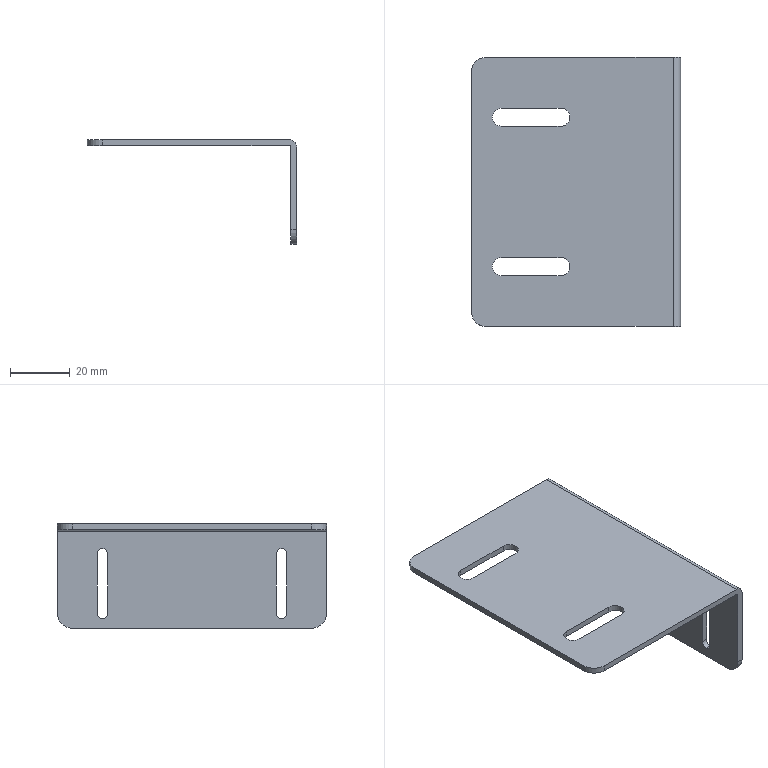Part | SolidWorks | features BaseBody 1 | 1 solid | 34 faces | box 70 x 90 x 35 mm | volume 17470 mm3 | cylinder 18 | plane 16 | commonest cylinder face diameters 3.5 x6 6 x6 10 x4 1 x1 5 x1
STEP:
#1=CARTESIAN_POINT('',(-63.,70.,0.));
#2=VERTEX_POINT('',#1);
#3=CARTESIAN_POINT('',(-60.,73.,0.));
#4=VERTEX_POINT('',#3);
#5=CARTESIAN_POINT('',(-60.,70.,0.));
#6=DIRECTION('',(0.,0.,-1.));
#7=DIRECTION('',(-1.,0.,0.));
#8=AXIS2_PLACEMENT_3D('',#5,#6,#7);
#9=CIRCLE('',#8,3.);
#10=EDGE_CURVE('',#2,#4,#9,.T.);
#11=ORIENTED_EDGE('',*,*,#10,.F.);
#12=CARTESIAN_POINT('',(-63.,70.,-2.));
#13=VERTEX_POINT('',#12);
#14=CARTESIAN_POINT('',(-63.,70.,8.));
#15=DIRECTION('',(0.,0.,-1.));
#16=VECTOR('',#15,1000.);
#17=LINE('',#14,#16);
#18=EDGE_CURVE('',#2,#13,#17,.T.);
#19=ORIENTED_EDGE('',*,*,#18,.T.);
#20=CARTESIAN_POINT('',(-60.,73.,-2.));
#21=VERTEX_POINT('',#20);
#22=CARTESIAN_POINT('',(-60.,70.,-2.));
#23=DIRECTION('',(0.,0.,1.));
#24=DIRECTION('',(-1.,0.,0.));
#25=AXIS2_PLACEMENT_3D('',#22,#23,#24);
#26=CIRCLE('',#25,3.);
#27=EDGE_CURVE('',#21,#13,#26,.T.);
#28=ORIENTED_EDGE('',*,*,#27,.F.);
#29=CARTESIAN_POINT('',(-60.,73.,8.));
#30=DIRECTION('',(0.,0.,1.));
#31=VECTOR('',#30,1000.);
#32=LINE('',#29,#31);
#33=EDGE_CURVE('',#21,#4,#32,.T.);
#34=ORIENTED_EDGE('',*,*,#33,.T.);
#35=EDGE_LOOP('',(#11,#19,#28,#34));
#36=FACE_OUTER_BOUND('',#35,.T.);
#37=CARTESIAN_POINT('',(-60.,70.,8.));
#38=DIRECTION('',(0.,0.,-1.));
#39=DIRECTION('',(-1.,0.,0.));
#40=AXIS2_PLACEMENT_3D('',#37,#38,#39);
#41=CYLINDRICAL_SURFACE('',#40,3.);
#42=ADVANCED_FACE('',(#36),#41,.F.);
#43=CARTESIAN_POINT('',(-63.,20.,0.));
#44=VERTEX_POINT('',#43);
#45=CARTESIAN_POINT('',(-60.,23.,0.));
#46=VERTEX_POINT('',#45);
#47=CARTESIAN_POINT('',(-60.,20.,0.));
#48=DIRECTION('',(0.,0.,-1.));
#49=DIRECTION('',(-1.,0.,0.));
#50=AXIS2_PLACEMENT_3D('',#47,#48,#49);
#51=CIRCLE('',#50,3.);
#52=EDGE_CURVE('',#44,#46,#51,.T.);
#53=ORIENTED_EDGE('',*,*,#52,.F.);
#54=CARTESIAN_POINT('',(-63.,20.,-2.));
#55=VERTEX_POINT('',#54);
#56=CARTESIAN_POINT('',(-63.,20.,8.));
#57=DIRECTION('',(0.,0.,-1.));
#58=VECTOR('',#57,1000.);
#59=LINE('',#56,#58);
#60=EDGE_CURVE('',#44,#55,#59,.T.);
#61=ORIENTED_EDGE('',*,*,#60,.T.);
#62=CARTESIAN_POINT('',(-60.,23.,-2.));
#63=VERTEX_POINT('',#62);
#64=CARTESIAN_POINT('',(-60.,20.,-2.));
#65=DIRECTION('',(0.,0.,1.));
#66=DIRECTION('',(-1.,0.,0.));
#67=AXIS2_PLACEMENT_3D('',#64,#65,#66);
#68=CIRCLE('',#67,3.);
#69=EDGE_CURVE('',#63,#55,#68,.T.);
#70=ORIENTED_EDGE('',*,*,#69,.F.);
#71=CARTESIAN_POINT('',(-60.,23.,8.));
#72=DIRECTION('',(0.,0.,1.));
#73=VECTOR('',#72,1000.);
#74=LINE('',#71,#73);
#75=EDGE_CURVE('',#63,#46,#74,.T.);
#76=ORIENTED_EDGE('',*,*,#75,.T.);
#77=EDGE_LOOP('',(#53,#61,#70,#76));
#78=FACE_OUTER_BOUND('',#77,.T.);
#79=CARTESIAN_POINT('',(-60.,20.,8.));
#80=DIRECTION('',(0.,0.,-1.));
#81=DIRECTION('',(-1.,0.,0.));
#82=AXIS2_PLACEMENT_3D('',#79,#80,#81);
#83=CYLINDRICAL_SURFACE('',#82,3.);
#84=ADVANCED_FACE('',(#78),#83,.F.);
#85=CARTESIAN_POINT('',(-2.,15.,-31.75));
#86=VERTEX_POINT('',#85);
#87=CARTESIAN_POINT('',(-2.,16.75,-30.));
#88=VERTEX_POINT('',#87);
#89=CARTESIAN_POINT('',(-2.,15.,-30.));
#90=DIRECTION('',(1.,0.,0.));
#91=DIRECTION('',(0.,0.,-1.));
#92=AXIS2_PLACEMENT_3D('',#89,#90,#91);
#93=CIRCLE('',#92,1.75);
#94=EDGE_CURVE('',#86,#88,#93,.T.);
#95=ORIENTED_EDGE('',*,*,#94,.F.);
#96=CARTESIAN_POINT('',(0.,15.,-31.75));
#97=VERTEX_POINT('',#96);
#98=CARTESIAN_POINT('',(-10.,15.,-31.75));
#99=DIRECTION('',(1.,0.,0.));
#100=VECTOR('',#99,1000.);
#101=LINE('',#98,#100);
#102=EDGE_CURVE('',#86,#97,#101,.T.);
#103=ORIENTED_EDGE('',*,*,#102,.T.);
#104=CARTESIAN_POINT('',(0.,16.75,-30.));
#105=VERTEX_POINT('',#104);
#106=CARTESIAN_POINT('',(0.,15.,-30.));
#107=DIRECTION('',(-1.,0.,0.));
#108=DIRECTION('',(0.,0.,-1.));
#109=AXIS2_PLACEMENT_3D('',#106,#107,#108);
#110=CIRCLE('',#109,1.75);
#111=EDGE_CURVE('',#105,#97,#110,.T.);
#112=ORIENTED_EDGE('',*,*,#111,.F.);
#113=CARTESIAN_POINT('',(-10.,16.75,-30.));
#114=DIRECTION('',(1.,0.,0.));
#115=VECTOR('',#114,1000.);
#116=LINE('',#113,#115);
#117=EDGE_CURVE('',#88,#105,#116,.T.);
#118=ORIENTED_EDGE('',*,*,#117,.F.);
#119=EDGE_LOOP('',(#95,#103,#112,#118));
#120=FACE_OUTER_BOUND('',#119,.T.);
#121=CARTESIAN_POINT('',(-10.,15.,-30.));
#122=DIRECTION('',(1.,0.,0.));
#123=DIRECTION('',(0.,0.,-1.));
#124=AXIS2_PLACEMENT_3D('',#121,#122,#123);
#125=CYLINDRICAL_SURFACE('',#124,1.75);
#126=ADVANCED_FACE('',(#120),#125,.F.);
#127=CARTESIAN_POINT('',(-2.,75.,-31.75));
#128=VERTEX_POINT('',#127);
#129=CARTESIAN_POINT('',(-2.,76.75,-30.));
#130=VERTEX_POINT('',#129);
#131=CARTESIAN_POINT('',(-2.,75.,-30.));
#132=DIRECTION('',(1.,0.,0.));
#133=DIRECTION('',(0.,0.,-1.));
#134=AXIS2_PLACEMENT_3D('',#131,#132,#133);
#135=CIRCLE('',#134,1.75);
#136=EDGE_CURVE('',#128,#130,#135,.T.);
#137=ORIENTED_EDGE('',*,*,#136,.F.);
#138=CARTESIAN_POINT('',(0.,75.,-31.75));
#139=VERTEX_POINT('',#138);
#140=CARTESIAN_POINT('',(-10.,75.,-31.75));
#141=DIRECTION('',(1.,0.,0.));
#142=VECTOR('',#141,1000.);
#143=LINE('',#140,#142);
#144=EDGE_CURVE('',#128,#139,#143,.T.);
#145=ORIENTED_EDGE('',*,*,#144,.T.);
#146=CARTESIAN_POINT('',(0.,76.75,-30.));
#147=VERTEX_POINT('',#146);
#148=CARTESIAN_POINT('',(0.,75.,-30.));
#149=DIRECTION('',(-1.,0.,0.));
#150=DIRECTION('',(0.,0.,-1.));
#151=AXIS2_PLACEMENT_3D('',#148,#149,#150);
#152=CIRCLE('',#151,1.75);
#153=EDGE_CURVE('',#147,#139,#152,.T.);
#154=ORIENTED_EDGE('',*,*,#153,.F.);
#155=CARTESIAN_POINT('',(-10.,76.75,-30.));
#156=DIRECTION('',(1.,0.,0.));
#157=VECTOR('',#156,1000.);
#158=LINE('',#155,#157);
#159=EDGE_CURVE('',#130,#147,#158,.T.);
#160=ORIENTED_EDGE('',*,*,#159,.F.);
#161=EDGE_LOOP('',(#137,#145,#154,#160));
#162=FACE_OUTER_BOUND('',#161,.T.);
#163=CARTESIAN_POINT('',(-10.,75.,-30.));
#164=DIRECTION('',(1.,0.,0.));
#165=DIRECTION('',(0.,0.,-1.));
#166=AXIS2_PLACEMENT_3D('',#163,#164,#165);
#167=CYLINDRICAL_SURFACE('',#166,1.75);
#168=ADVANCED_FACE('',(#162),#167,.F.);
#169=CARTESIAN_POINT('',(-65.,0.,0.));
#170=VERTEX_POINT('',#169);
#171=CARTESIAN_POINT('',(-2.5,0.,0.));
#172=VERTEX_POINT('',#171);
#173=CARTESIAN_POINT('',(0.,0.,0.));
#174=DIRECTION('',(1.,0.,0.));
#175=VECTOR('',#174,1000.);
#176=LINE('',#173,#175);
#177=EDGE_CURVE('',#170,#172,#176,.T.);
#178=ORIENTED_EDGE('',*,*,#177,.T.);
#179=CARTESIAN_POINT('',(-2.5,90.,0.));
#180=VERTEX_POINT('',#179);
#181=CARTESIAN_POINT('',(-2.5,90.,0.));
#182=DIRECTION('',(0.,1.,0.));
#183=VECTOR('',#182,1000.);
#184=LINE('',#181,#183);
#185=EDGE_CURVE('',#172,#180,#184,.T.);
#186=ORIENTED_EDGE('',*,*,#185,.T.);
#187=CARTESIAN_POINT('',(-65.,90.,0.));
#188=VERTEX_POINT('',#187);
#189=CARTESIAN_POINT('',(0.,90.,0.));
#190=DIRECTION('',(-1.,0.,0.));
#191=VECTOR('',#190,1000.);
#192=LINE('',#189,#191);
#193=EDGE_CURVE('',#180,#188,#192,.T.);
#194=ORIENTED_EDGE('',*,*,#193,.T.);
#195=CARTESIAN_POINT('',(-70.,85.,0.));
#196=VERTEX_POINT('',#195);
#197=CARTESIAN_POINT('',(-65.,85.,0.));
#198=DIRECTION('',(0.,0.,1.));
#199=DIRECTION('',(-1.,0.,0.));
#200=AXIS2_PLACEMENT_3D('',#197,#198,#199);
#201=CIRCLE('',#200,5.);
#202=EDGE_CURVE('',#188,#196,#201,.T.);
#203=ORIENTED_EDGE('',*,*,#202,.T.);
#204=CARTESIAN_POINT('',(-70.,5.,0.));
#205=VERTEX_POINT('',#204);
#206=CARTESIAN_POINT('',(-70.,90.,0.));
#207=DIRECTION('',(0.,-1.,0.));
#208=VECTOR('',#207,1000.);
#209=LINE('',#206,#208);
#210=EDGE_CURVE('',#196,#205,#209,.T.);
#211=ORIENTED_EDGE('',*,*,#210,.T.);
#212=CARTESIAN_POINT('',(-65.,5.,0.));
#213=DIRECTION('',(0.,0.,1.));
#214=DIRECTION('',(1.,0.,0.));
#215=AXIS2_PLACEMENT_3D('',#212,#213,#214);
#216=CIRCLE('',#215,5.);
#217=EDGE_CURVE('',#205,#170,#216,.T.);
#218=ORIENTED_EDGE('',*,*,#217,.T.);
#219=EDGE_LOOP('',(#178,#186,#194,#203,#211,#218));
#220=FACE_OUTER_BOUND('',#219,.T.);
#221=CARTESIAN_POINT('',(-60.,67.,0.));
#222=VERTEX_POINT('',#221);
#223=CARTESIAN_POINT('',(-60.,70.,0.));
#224=DIRECTION('',(0.,0.,-1.));
#225=DIRECTION('',(-1.,0.,0.));
#226=AXIS2_PLACEMENT_3D('',#223,#224,#225);
#227=CIRCLE('',#226,3.);
#228=EDGE_CURVE('',#222,#2,#227,.T.);
#229=ORIENTED_EDGE('',*,*,#228,.T.);
#230=ORIENTED_EDGE('',*,*,#10,.T.);
#231=CARTESIAN_POINT('',(-40.,73.,0.));
#232=VERTEX_POINT('',#231);
#233=CARTESIAN_POINT('',(0.,73.,0.));
#234=DIRECTION('',(1.,0.,0.));
#235=VECTOR('',#234,1000.);
#236=LINE('',#233,#235);
#237=EDGE_CURVE('',#4,#232,#236,.T.);
#238=ORIENTED_EDGE('',*,*,#237,.T.);
#239=CARTESIAN_POINT('',(-40.,67.,0.));
#240=VERTEX_POINT('',#239);
#241=CARTESIAN_POINT('',(-40.,70.,0.));
#242=DIRECTION('',(0.,0.,-1.));
#243=DIRECTION('',(-1.,0.,0.));
#244=AXIS2_PLACEMENT_3D('',#241,#242,#243);
#245=CIRCLE('',#244,3.);
#246=EDGE_CURVE('',#232,#240,#245,.T.);
#247=ORIENTED_EDGE('',*,*,#246,.T.);
#248=CARTESIAN_POINT('',(0.,67.,0.));
#249=DIRECTION('',(-1.,0.,0.));
#250=VECTOR('',#249,1000.);
#251=LINE('',#248,#250);
#252=EDGE_CURVE('',#240,#222,#251,.T.);
#253=ORIENTED_EDGE('',*,*,#252,.T.);
#254=EDGE_LOOP('',(#229,#230,#238,#247,#253));
#255=FACE_BOUND('',#254,.T.);
#256=CARTESIAN_POINT('',(-60.,17.,0.));
#257=VERTEX_POINT('',#256);
#258=CARTESIAN_POINT('',(-60.,20.,0.));
#259=DIRECTION('',(0.,0.,-1.));
#260=DIRECTION('',(-1.,0.,0.));
#261=AXIS2_PLACEMENT_3D('',#258,#259,#260);
#262=CIRCLE('',#261,3.);
#263=EDGE_CURVE('',#257,#44,#262,.T.);
#264=ORIENTED_EDGE('',*,*,#263,.T.);
#265=ORIENTED_EDGE('',*,*,#52,.T.);
#266=CARTESIAN_POINT('',(-40.,23.,0.));
#267=VERTEX_POINT('',#266);
#268=CARTESIAN_POINT('',(0.,23.,0.));
#269=DIRECTION('',(1.,0.,0.));
#270=VECTOR('',#269,1000.);
#271=LINE('',#268,#270);
#272=EDGE_CURVE('',#46,#267,#271,.T.);
#273=ORIENTED_EDGE('',*,*,#272,.T.);
#274=CARTESIAN_POINT('',(-40.,17.,0.));
#275=VERTEX_POINT('',#274);
#276=CARTESIAN_POINT('',(-40.,20.,0.));
#277=DIRECTION('',(0.,0.,-1.));
#278=DIRECTION('',(-1.,0.,0.));
#279=AXIS2_PLACEMENT_3D('',#276,#277,#278);
#280=CIRCLE('',#279,3.);
#281=EDGE_CURVE('',#267,#275,#280,.T.);
#282=ORIENTED_EDGE('',*,*,#281,.T.);
#283=CARTESIAN_POINT('',(0.,17.,0.));
#284=DIRECTION('',(-1.,0.,0.));
#285=VECTOR('',#284,1000.);
#286=LINE('',#283,#285);
#287=EDGE_CURVE('',#275,#257,#286,.T.);
#288=ORIENTED_EDGE('',*,*,#287,.T.);
#289=EDGE_LOOP('',(#264,#265,#273,#282,#288));
#290=FACE_BOUND('',#289,.T.);
#291=CARTESIAN_POINT('',(0.,90.,0.));
#292=DIRECTION('',(0.,0.,1.));
#293=DIRECTION('',(1.,0.,0.));
#294=AXIS2_PLACEMENT_3D('',#291,#292,#293);
#295=PLANE('',#294);
#296=ADVANCED_FACE('',(#220,#255,#290),#295,.T.);
#297=CARTESIAN_POINT('',(0.,90.,-2.5));
#298=VERTEX_POINT('',#297);
#299=CARTESIAN_POINT('',(-2.5,90.,-2.5));
#300=DIRECTION('',(0.,-1.,0.));
#301=DIRECTION('',(0.,0.,-1.));
#302=AXIS2_PLACEMENT_3D('',#299,#300,#301);
#303=CIRCLE('',#302,2.5);
#304=EDGE_CURVE('',#298,#180,#303,.T.);
#305=ORIENTED_EDGE('',*,*,#304,.T.);
#306=ORIENTED_EDGE('',*,*,#185,.F.);
#307=CARTESIAN_POINT('',(0.,0.,-2.5));
#308=VERTEX_POINT('',#307);
#309=CARTESIAN_POINT('',(-2.5,0.,-2.5));
#310=DIRECTION('',(0.,1.,0.));
#311=DIRECTION('',(0.,0.,-1.));
#312=AXIS2_PLACEMENT_3D('',#309,#310,#311);
#313=CIRCLE('',#312,2.5);
#314=EDGE_CURVE('',#172,#308,#313,.T.);
#315=ORIENTED_EDGE('',*,*,#314,.T.);
#316=CARTESIAN_POINT('',(0.,90.,-2.5));
#317=DIRECTION('',(0.,1.,0.));
#318=VECTOR('',#317,1000.);
#319=LINE('',#316,#318);
#320=EDGE_CURVE('',#308,#298,#319,.T.);
#321=ORIENTED_EDGE('',*,*,#320,.T.);
#322=EDGE_LOOP('',(#305,#306,#315,#321));
#323=FACE_OUTER_BOUND('',#322,.T.);
#324=CARTESIAN_POINT('',(-2.5,90.,-2.5));
#325=DIRECTION('',(0.,-1.,0.));
#326=DIRECTION('',(0.,0.,-1.));
#327=AXIS2_PLACEMENT_3D('',#324,#325,#326);
#328=CYLINDRICAL_SURFACE('',#327,2.5);
#329=ADVANCED_FACE('',(#323),#328,.T.);
#330=CARTESIAN_POINT('',(-65.,0.,-2.));
#331=VERTEX_POINT('',#330);
#332=CARTESIAN_POINT('',(-65.,0.,-2.5));
#333=DIRECTION('',(0.,0.,1.));
#334=VECTOR('',#333,1000.);
#335=LINE('',#332,#334);
#336=EDGE_CURVE('',#331,#170,#335,.T.);
#337=ORIENTED_EDGE('',*,*,#336,.F.);
#338=CARTESIAN_POINT('',(-2.5,0.,-2.));
#339=VERTEX_POINT('',#338);
#340=CARTESIAN_POINT('',(-2.5,0.,-2.));
#341=DIRECTION('',(-1.,0.,0.));
#342=VECTOR('',#341,1000.);
#343=LINE('',#340,#342);
#344=EDGE_CURVE('',#339,#331,#343,.T.);
#345=ORIENTED_EDGE('',*,*,#344,.F.);
#346=CARTESIAN_POINT('',(-2.,0.,-2.5));
#347=VERTEX_POINT('',#346);
#348=CARTESIAN_POINT('',(-2.5,0.,-2.5));
#349=DIRECTION('',(0.,1.,0.));
#350=DIRECTION('',(0.,0.,-1.));
#351=AXIS2_PLACEMENT_3D('',#348,#349,#350);
#352=CIRCLE('',#351,0.5);
#353=EDGE_CURVE('',#339,#347,#352,.T.);
#354=ORIENTED_EDGE('',*,*,#353,.T.);
#355=CARTESIAN_POINT('',(-2.,0.,-30.));
#356=VERTEX_POINT('',#355);
#357=CARTESIAN_POINT('',(-2.,0.,-2.));
#358=DIRECTION('',(0.,0.,-1.));
#359=VECTOR('',#358,1000.);
#360=LINE('',#357,#359);
#361=EDGE_CURVE('',#347,#356,#360,.T.);
#362=ORIENTED_EDGE('',*,*,#361,.T.);
#363=CARTESIAN_POINT('',(0.,0.,-30.));
#364=VERTEX_POINT('',#363);
#365=CARTESIAN_POINT('',(-2.5,0.,-30.));
#366=DIRECTION('',(-1.,0.,0.));
#367=VECTOR('',#366,1000.);
#368=LINE('',#365,#367);
#369=EDGE_CURVE('',#364,#356,#368,.T.);
#370=ORIENTED_EDGE('',*,*,#369,.F.);
#371=CARTESIAN_POINT('',(0.,0.,-35.));
#372=DIRECTION('',(0.,0.,-1.));
#373=VECTOR('',#372,1000.);
#374=LINE('',#371,#373);
#375=EDGE_CURVE('',#308,#364,#374,.T.);
#376=ORIENTED_EDGE('',*,*,#375,.F.);
#377=ORIENTED_EDGE('',*,*,#314,.F.);
#378=ORIENTED_EDGE('',*,*,#177,.F.);
#379=EDGE_LOOP('',(#337,#345,#354,#362,#370,#376,#377,#378));
#380=FACE_OUTER_BOUND('',#379,.T.);
#381=CARTESIAN_POINT('',(-2.5,0.,-2.5));
#382=DIRECTION('',(0.,1.,0.));
#383=DIRECTION('',(0.,0.,1.));
#384=AXIS2_PLACEMENT_3D('',#381,#382,#383);
#385=PLANE('',#384);
#386=ADVANCED_FACE('',(#380),#385,.F.);
#387=CARTESIAN_POINT('',(-70.,5.,-2.));
#388=VERTEX_POINT('',#387);
#389=CARTESIAN_POINT('',(-65.,5.,-2.));
#390=DIRECTION('',(0.,0.,1.));
#391=DIRECTION('',(1.,0.,0.));
#392=AXIS2_PLACEMENT_3D('',#389,#390,#391);
#393=CIRCLE('',#392,5.);
#394=EDGE_CURVE('',#388,#331,#393,.T.);
#395=ORIENTED_EDGE('',*,*,#394,.T.);
#396=ORIENTED_EDGE('',*,*,#336,.T.);
#397=ORIENTED_EDGE('',*,*,#217,.F.);
#398=CARTESIAN_POINT('',(-70.,5.,-2.5));
#399=DIRECTION('',(0.,0.,-1.));
#400=VECTOR('',#399,1000.);
#401=LINE('',#398,#400);
#402=EDGE_CURVE('',#205,#388,#401,.T.);
#403=ORIENTED_EDGE('',*,*,#402,.T.);
#404=EDGE_LOOP('',(#395,#396,#397,#403));
#405=FACE_OUTER_BOUND('',#404,.T.);
#406=CARTESIAN_POINT('',(-65.,5.,-2.5));
#407=DIRECTION('',(0.,0.,1.));
#408=DIRECTION('',(1.,0.,0.));
#409=AXIS2_PLACEMENT_3D('',#406,#407,#408);
#410=CYLINDRICAL_SURFACE('',#409,5.);
#411=ADVANCED_FACE('',(#405),#410,.T.);
#412=CARTESIAN_POINT('',(-70.,85.,-2.));
#413=VERTEX_POINT('',#412);
#414=CARTESIAN_POINT('',(-70.,90.,-2.));
#415=DIRECTION('',(0.,-1.,0.));
#416=VECTOR('',#415,1000.);
#417=LINE('',#414,#416);
#418=EDGE_CURVE('',#413,#388,#417,.T.);
#419=ORIENTED_EDGE('',*,*,#418,.T.);
#420=ORIENTED_EDGE('',*,*,#402,.F.);
#421=ORIENTED_EDGE('',*,*,#210,.F.);
#422=CARTESIAN_POINT('',(-70.,85.,0.));
#423=DIRECTION('',(0.,0.,-1.));
#424=VECTOR('',#423,1000.);
#425=LINE('',#422,#424);
#426=EDGE_CURVE('',#196,#413,#425,.T.);
#427=ORIENTED_EDGE('',*,*,#426,.T.);
#428=EDGE_LOOP('',(#419,#420,#421,#427));
#429=FACE_OUTER_BOUND('',#428,.T.);
#430=CARTESIAN_POINT('',(-70.,90.,0.));
#431=DIRECTION('',(-1.,0.,0.));
#432=DIRECTION('',(0.,0.,1.));
#433=AXIS2_PLACEMENT_3D('',#430,#431,#432);
#434=PLANE('',#433);
#435=ADVANCED_FACE('',(#429),#434,.T.);
#436=CARTESIAN_POINT('',(-65.,90.,-2.));
#437=VERTEX_POINT('',#436);
#438=CARTESIAN_POINT('',(-65.,85.,-2.));
#439=DIRECTION('',(0.,0.,1.));
#440=DIRECTION('',(-1.,0.,0.));
#441=AXIS2_PLACEMENT_3D('',#438,#439,#440);
#442=CIRCLE('',#441,5.);
#443=EDGE_CURVE('',#437,#413,#442,.T.);
#444=ORIENTED_EDGE('',*,*,#443,.T.);
#445=ORIENTED_EDGE('',*,*,#426,.F.);
#446=ORIENTED_EDGE('',*,*,#202,.F.);
#447=CARTESIAN_POINT('',(-65.,90.,0.));
#448=DIRECTION('',(0.,0.,-1.));
#449=VECTOR('',#448,1000.);
#450=LINE('',#447,#449);
#451=EDGE_CURVE('',#188,#437,#450,.T.);
#452=ORIENTED_EDGE('',*,*,#451,.T.);
#453=EDGE_LOOP('',(#444,#445,#446,#452));
#454=FACE_OUTER_BOUND('',#453,.T.);
#455=CARTESIAN_POINT('',(-65.,85.,0.));
#456=DIRECTION('',(0.,0.,-1.));
#457=DIRECTION('',(-1.,0.,0.));
#458=AXIS2_PLACEMENT_3D('',#455,#456,#457);
#459=CYLINDRICAL_SURFACE('',#458,5.);
#460=ADVANCED_FACE('',(#454),#459,.T.);
#461=ORIENTED_EDGE('',*,*,#193,.F.);
#462=ORIENTED_EDGE('',*,*,#304,.F.);
#463=CARTESIAN_POINT('',(0.,90.,-30.));
#464=VERTEX_POINT('',#463);
#465=CARTESIAN_POINT('',(0.,90.,-35.));
#466=DIRECTION('',(0.,0.,1.));
#467=VECTOR('',#466,1000.);
#468=LINE('',#465,#467);
#469=EDGE_CURVE('',#464,#298,#468,.T.);
#470=ORIENTED_EDGE('',*,*,#469,.F.);
#471=CARTESIAN_POINT('',(-2.,90.,-30.));
#472=VERTEX_POINT('',#471);
#473=CARTESIAN_POINT('',(-2.5,90.,-30.));
#474=DIRECTION('',(-1.,0.,0.));
#475=VECTOR('',#474,1000.);
#476=LINE('',#473,#475);
#477=EDGE_CURVE('',#464,#472,#476,.T.);
#478=ORIENTED_EDGE('',*,*,#477,.T.);
#479=CARTESIAN_POINT('',(-2.,90.,-2.5));
#480=VERTEX_POINT('',#479);
#481=CARTESIAN_POINT('',(-2.,90.,-2.5));
#482=DIRECTION('',(0.,0.,1.));
#483=VECTOR('',#482,1000.);
#484=LINE('',#481,#483);
#485=EDGE_CURVE('',#472,#480,#484,.T.);
#486=ORIENTED_EDGE('',*,*,#485,.T.);
#487=CARTESIAN_POINT('',(-2.5,90.,-2.));
#488=VERTEX_POINT('',#487);
#489=CARTESIAN_POINT('',(-2.5,90.,-2.5));
#490=DIRECTION('',(0.,-1.,0.));
#491=DIRECTION('',(0.,0.,-1.));
#492=AXIS2_PLACEMENT_3D('',#489,#490,#491);
#493=CIRCLE('',#492,0.5);
#494=EDGE_CURVE('',#480,#488,#493,.T.);
#495=ORIENTED_EDGE('',*,*,#494,.T.);
#496=CARTESIAN_POINT('',(-2.,90.,-2.));
#497=DIRECTION('',(-1.,0.,0.));
#498=VECTOR('',#497,1000.);
#499=LINE('',#496,#498);
#500=EDGE_CURVE('',#488,#437,#499,.T.);
#501=ORIENTED_EDGE('',*,*,#500,.T.);
#502=ORIENTED_EDGE('',*,*,#451,.F.);
#503=EDGE_LOOP('',(#461,#462,#470,#478,#486,#495,#501,#502));
#504=FACE_OUTER_BOUND('',#503,.T.);
#505=CARTESIAN_POINT('',(-2.,90.,-2.5));
#506=DIRECTION('',(0.,1.,0.));
#507=DIRECTION('',(0.,0.,1.));
#508=AXIS2_PLACEMENT_3D('',#505,#506,#507);
#509=PLANE('',#508);
#510=ADVANCED_FACE('',(#504),#509,.T.);
#511=ORIENTED_EDGE('',*,*,#33,.F.);
#512=CARTESIAN_POINT('',(-40.,73.,-2.));
#513=VERTEX_POINT('',#512);
#514=CARTESIAN_POINT('',(-40.,73.,-2.));
#515=DIRECTION('',(-1.,0.,0.));
#516=VECTOR('',#515,1000.);
#517=LINE('',#514,#516);
#518=EDGE_CURVE('',#513,#21,#517,.T.);
#519=ORIENTED_EDGE('',*,*,#518,.F.);
#520=CARTESIAN_POINT('',(-40.,73.,8.));
#521=DIRECTION('',(0.,0.,-1.));
#522=VECTOR('',#521,1000.);
#523=LINE('',#520,#522);
#524=EDGE_CURVE('',#232,#513,#523,.T.);
#525=ORIENTED_EDGE('',*,*,#524,.F.);
#526=ORIENTED_EDGE('',*,*,#237,.F.);
#527=EDGE_LOOP('',(#511,#519,#525,#526));
#528=FACE_OUTER_BOUND('',#527,.T.);
#529=CARTESIAN_POINT('',(-40.,73.,8.));
#530=DIRECTION('',(0.,1.,0.));
#531=DIRECTION('',(0.,0.,1.));
#532=AXIS2_PLACEMENT_3D('',#529,#530,#531);
#533=PLANE('',#532);
#534=ADVANCED_FACE('',(#528),#533,.F.);
#535=ORIENTED_EDGE('',*,*,#18,.F.);
#536=ORIENTED_EDGE('',*,*,#228,.F.);
#537=CARTESIAN_POINT('',(-60.,67.,-2.));
#538=VERTEX_POINT('',#537);
#539=CARTESIAN_POINT('',(-60.,67.,8.));
#540=DIRECTION('',(0.,0.,1.));
#541=VECTOR('',#540,1000.);
#542=LINE('',#539,#541);
#543=EDGE_CURVE('',#538,#222,#542,.T.);
#544=ORIENTED_EDGE('',*,*,#543,.F.);
#545=CARTESIAN_POINT('',(-60.,70.,-2.));
#546=DIRECTION('',(0.,0.,1.));
#547=DIRECTION('',(-1.,0.,0.));
#548=AXIS2_PLACEMENT_3D('',#545,#546,#547);
#549=CIRCLE('',#548,3.);
#550=EDGE_CURVE('',#13,#538,#549,.T.);
#551=ORIENTED_EDGE('',*,*,#550,.F.);
#552=EDGE_LOOP('',(#535,#536,#544,#551));
#553=FACE_OUTER_BOUND('',#552,.T.);
#554=CARTESIAN_POINT('',(-60.,70.,8.));
#555=DIRECTION('',(0.,0.,-1.));
#556=DIRECTION('',(-1.,0.,0.));
#557=AXIS2_PLACEMENT_3D('',#554,#555,#556);
#558=CYLINDRICAL_SURFACE('',#557,3.);
#559=ADVANCED_FACE('',(#553),#558,.F.);
#560=CARTESIAN_POINT('',(-40.,67.,-2.));
#561=VERTEX_POINT('',#560);
#562=CARTESIAN_POINT('',(-40.,67.,8.));
#563=DIRECTION('',(0.,0.,1.));
#564=VECTOR('',#563,1000.);
#565=LINE('',#562,#564);
#566=EDGE_CURVE('',#561,#240,#565,.T.);
#567=ORIENTED_EDGE('',*,*,#566,.F.);
#568=CARTESIAN_POINT('',(-40.,67.,-2.));
#569=DIRECTION('',(1.,0.,0.));
#570=VECTOR('',#569,1000.);
#571=LINE('',#568,#570);
#572=EDGE_CURVE('',#538,#561,#571,.T.);
#573=ORIENTED_EDGE('',*,*,#572,.F.);
#574=ORIENTED_EDGE('',*,*,#543,.T.);
#575=ORIENTED_EDGE('',*,*,#252,.F.);
#576=EDGE_LOOP('',(#567,#573,#574,#575));
#577=FACE_OUTER_BOUND('',#576,.T.);
#578=CARTESIAN_POINT('',(-40.,67.,8.));
#579=DIRECTION('',(0.,-1.,0.));
#580=DIRECTION('',(0.,0.,-1.));
#581=AXIS2_PLACEMENT_3D('',#578,#579,#580);
#582=PLANE('',#581);
#583=ADVANCED_FACE('',(#577),#582,.F.);
#584=ORIENTED_EDGE('',*,*,#524,.T.);
#585=CARTESIAN_POINT('',(-40.,70.,-2.));
#586=DIRECTION('',(0.,0.,1.));
#587=DIRECTION('',(-1.,0.,0.));
#588=AXIS2_PLACEMENT_3D('',#585,#586,#587);
#589=CIRCLE('',#588,3.);
#590=EDGE_CURVE('',#561,#513,#589,.T.);
#591=ORIENTED_EDGE('',*,*,#590,.F.);
#592=ORIENTED_EDGE('',*,*,#566,.T.);
#593=ORIENTED_EDGE('',*,*,#246,.F.);
#594=EDGE_LOOP('',(#584,#591,#592,#593));
#595=FACE_OUTER_BOUND('',#594,.T.);
#596=CARTESIAN_POINT('',(-40.,70.,8.));
#597=DIRECTION('',(0.,0.,-1.));
#598=DIRECTION('',(-1.,0.,0.));
#599=AXIS2_PLACEMENT_3D('',#596,#597,#598);
#600=CYLINDRICAL_SURFACE('',#599,3.);
#601=ADVANCED_FACE('',(#595),#600,.F.);
#602=ORIENTED_EDGE('',*,*,#75,.F.);
#603=CARTESIAN_POINT('',(-40.,23.,-2.));
#604=VERTEX_POINT('',#603);
#605=CARTESIAN_POINT('',(-40.,23.,-2.));
#606=DIRECTION('',(-1.,0.,0.));
#607=VECTOR('',#606,1000.);
#608=LINE('',#605,#607);
#609=EDGE_CURVE('',#604,#63,#608,.T.);
#610=ORIENTED_EDGE('',*,*,#609,.F.);
#611=CARTESIAN_POINT('',(-40.,23.,8.));
#612=DIRECTION('',(0.,0.,-1.));
#613=VECTOR('',#612,1000.);
#614=LINE('',#611,#613);
#615=EDGE_CURVE('',#267,#604,#614,.T.);
#616=ORIENTED_EDGE('',*,*,#615,.F.);
#617=ORIENTED_EDGE('',*,*,#272,.F.);
#618=EDGE_LOOP('',(#602,#610,#616,#617));
#619=FACE_OUTER_BOUND('',#618,.T.);
#620=CARTESIAN_POINT('',(-40.,23.,8.));
#621=DIRECTION('',(0.,1.,0.));
#622=DIRECTION('',(0.,0.,1.));
#623=AXIS2_PLACEMENT_3D('',#620,#621,#622);
#624=PLANE('',#623);
#625=ADVANCED_FACE('',(#619),#624,.F.);
#626=ORIENTED_EDGE('',*,*,#60,.F.);
#627=ORIENTED_EDGE('',*,*,#263,.F.);
#628=CARTESIAN_POINT('',(-60.,17.,-2.));
#629=VERTEX_POINT('',#628);
#630=CARTESIAN_POINT('',(-60.,17.,8.));
#631=DIRECTION('',(0.,0.,1.));
#632=VECTOR('',#631,1000.);
#633=LINE('',#630,#632);
#634=EDGE_CURVE('',#629,#257,#633,.T.);
#635=ORIENTED_EDGE('',*,*,#634,.F.);
#636=CARTESIAN_POINT('',(-60.,20.,-2.));
#637=DIRECTION('',(0.,0.,1.));
#638=DIRECTION('',(-1.,0.,0.));
#639=AXIS2_PLACEMENT_3D('',#636,#637,#638);
#640=CIRCLE('',#639,3.);
#641=EDGE_CURVE('',#55,#629,#640,.T.);
#642=ORIENTED_EDGE('',*,*,#641,.F.);
#643=EDGE_LOOP('',(#626,#627,#635,#642));
#644=FACE_OUTER_BOUND('',#643,.T.);
#645=CARTESIAN_POINT('',(-60.,20.,8.));
#646=DIRECTION('',(0.,0.,-1.));
#647=DIRECTION('',(-1.,0.,0.));
#648=AXIS2_PLACEMENT_3D('',#645,#646,#647);
#649=CYLINDRICAL_SURFACE('',#648,3.);
#650=ADVANCED_FACE('',(#644),#649,.F.);
#651=CARTESIAN_POINT('',(-40.,17.,-2.));
#652=VERTEX_POINT('',#651);
#653=CARTESIAN_POINT('',(-40.,17.,8.));
#654=DIRECTION('',(0.,0.,1.));
#655=VECTOR('',#654,1000.);
#656=LINE('',#653,#655);
#657=EDGE_CURVE('',#652,#275,#656,.T.);
#658=ORIENTED_EDGE('',*,*,#657,.F.);
#659=CARTESIAN_POINT('',(-40.,17.,-2.));
#660=DIRECTION('',(1.,0.,0.));
#661=VECTOR('',#660,1000.);
#662=LINE('',#659,#661);
#663=EDGE_CURVE('',#629,#652,#662,.T.);
#664=ORIENTED_EDGE('',*,*,#663,.F.);
#665=ORIENTED_EDGE('',*,*,#634,.T.);
#666=ORIENTED_EDGE('',*,*,#287,.F.);
#667=EDGE_LOOP('',(#658,#664,#665,#666));
#668=FACE_OUTER_BOUND('',#667,.T.);
#669=CARTESIAN_POINT('',(-40.,17.,8.));
#670=DIRECTION('',(0.,-1.,0.));
#671=DIRECTION('',(0.,0.,-1.));
#672=AXIS2_PLACEMENT_3D('',#669,#670,#671);
#673=PLANE('',#672);
#674=ADVANCED_FACE('',(#668),#673,.F.);
#675=ORIENTED_EDGE('',*,*,#615,.T.);
#676=CARTESIAN_POINT('',(-40.,20.,-2.));
#677=DIRECTION('',(0.,0.,1.));
#678=DIRECTION('',(-1.,0.,0.));
#679=AXIS2_PLACEMENT_3D('',#676,#677,#678);
#680=CIRCLE('',#679,3.);
#681=EDGE_CURVE('',#652,#604,#680,.T.);
#682=ORIENTED_EDGE('',*,*,#681,.F.);
#683=ORIENTED_EDGE('',*,*,#657,.T.);
#684=ORIENTED_EDGE('',*,*,#281,.F.);
#685=EDGE_LOOP('',(#675,#682,#683,#684));
#686=FACE_OUTER_BOUND('',#685,.T.);
#687=CARTESIAN_POINT('',(-40.,20.,8.));
#688=DIRECTION('',(0.,0.,-1.));
#689=DIRECTION('',(-1.,0.,0.));
#690=AXIS2_PLACEMENT_3D('',#687,#688,#689);
#691=CYLINDRICAL_SURFACE('',#690,3.);
#692=ADVANCED_FACE('',(#686),#691,.F.);
#693=ORIENTED_EDGE('',*,*,#469,.T.);
#694=ORIENTED_EDGE('',*,*,#320,.F.);
#695=ORIENTED_EDGE('',*,*,#375,.T.);
#696=CARTESIAN_POINT('',(0.,5.,-35.));
#697=VERTEX_POINT('',#696);
#698=CARTESIAN_POINT('',(0.,5.,-30.));
#699=DIRECTION('',(1.,0.,0.));
#700=DIRECTION('',(0.,0.,-1.));
#701=AXIS2_PLACEMENT_3D('',#698,#699,#700);
#702=CIRCLE('',#701,5.);
#703=EDGE_CURVE('',#364,#697,#702,.T.);
#704=ORIENTED_EDGE('',*,*,#703,.T.);
#705=CARTESIAN_POINT('',(0.,85.,-35.));
#706=VERTEX_POINT('',#705);
#707=CARTESIAN_POINT('',(0.,90.,-35.));
#708=DIRECTION('',(0.,1.,0.));
#709=VECTOR('',#708,1000.);
#710=LINE('',#707,#709);
#711=EDGE_CURVE('',#697,#706,#710,.T.);
#712=ORIENTED_EDGE('',*,*,#711,.T.);
#713=CARTESIAN_POINT('',(0.,85.,-30.));
#714=DIRECTION('',(1.,0.,0.));
#715=DIRECTION('',(0.,0.,-1.));
#716=AXIS2_PLACEMENT_3D('',#713,#714,#715);
#717=CIRCLE('',#716,5.);
#718=EDGE_CURVE('',#706,#464,#717,.T.);
#719=ORIENTED_EDGE('',*,*,#718,.T.);
#720=EDGE_LOOP('',(#693,#694,#695,#704,#712,#719));
#721=FACE_OUTER_BOUND('',#720,.T.);
#722=ORIENTED_EDGE('',*,*,#111,.T.);
#723=CARTESIAN_POINT('',(0.,13.25,-30.));
#724=VERTEX_POINT('',#723);
#725=CARTESIAN_POINT('',(0.,15.,-30.));
#726=DIRECTION('',(-1.,0.,0.));
#727=DIRECTION('',(0.,0.,-1.));
#728=AXIS2_PLACEMENT_3D('',#725,#726,#727);
#729=CIRCLE('',#728,1.75);
#730=EDGE_CURVE('',#97,#724,#729,.T.);
#731=ORIENTED_EDGE('',*,*,#730,.T.);
#732=CARTESIAN_POINT('',(0.,13.25,-10.));
#733=VERTEX_POINT('',#732);
#734=CARTESIAN_POINT('',(0.,13.25,-35.));
#735=DIRECTION('',(0.,0.,1.));
#736=VECTOR('',#735,1000.);
#737=LINE('',#734,#736);
#738=EDGE_CURVE('',#724,#733,#737,.T.);
#739=ORIENTED_EDGE('',*,*,#738,.T.);
#740=CARTESIAN_POINT('',(0.,16.75,-10.));
#741=VERTEX_POINT('',#740);
#742=CARTESIAN_POINT('',(0.,15.,-10.));
#743=DIRECTION('',(-1.,0.,0.));
#744=DIRECTION('',(0.,0.,-1.));
#745=AXIS2_PLACEMENT_3D('',#742,#743,#744);
#746=CIRCLE('',#745,1.75);
#747=EDGE_CURVE('',#733,#741,#746,.T.);
#748=ORIENTED_EDGE('',*,*,#747,.T.);
#749=CARTESIAN_POINT('',(0.,16.75,-35.));
#750=DIRECTION('',(0.,0.,-1.));
#751=VECTOR('',#750,1000.);
#752=LINE('',#749,#751);
#753=EDGE_CURVE('',#741,#105,#752,.T.);
#754=ORIENTED_EDGE('',*,*,#753,.T.);
#755=EDGE_LOOP('',(#722,#731,#739,#748,#754));
#756=FACE_BOUND('',#755,.T.);
#757=ORIENTED_EDGE('',*,*,#153,.T.);
#758=CARTESIAN_POINT('',(0.,73.25,-30.));
#759=VERTEX_POINT('',#758);
#760=CARTESIAN_POINT('',(0.,75.,-30.));
#761=DIRECTION('',(-1.,0.,0.));
#762=DIRECTION('',(0.,0.,-1.));
#763=AXIS2_PLACEMENT_3D('',#760,#761,#762);
#764=CIRCLE('',#763,1.75);
#765=EDGE_CURVE('',#139,#759,#764,.T.);
#766=ORIENTED_EDGE('',*,*,#765,.T.);
#767=CARTESIAN_POINT('',(0.,73.25,-10.));
#768=VERTEX_POINT('',#767);
#769=CARTESIAN_POINT('',(0.,73.25,-35.));
#770=DIRECTION('',(0.,0.,1.));
#771=VECTOR('',#770,1000.);
#772=LINE('',#769,#771);
#773=EDGE_CURVE('',#759,#768,#772,.T.);
#774=ORIENTED_EDGE('',*,*,#773,.T.);
#775=CARTESIAN_POINT('',(0.,76.75,-10.));
#776=VERTEX_POINT('',#775);
#777=CARTESIAN_POINT('',(0.,75.,-10.));
#778=DIRECTION('',(-1.,0.,0.));
#779=DIRECTION('',(0.,0.,-1.));
#780=AXIS2_PLACEMENT_3D('',#777,#778,#779);
#781=CIRCLE('',#780,1.75);
#782=EDGE_CURVE('',#768,#776,#781,.T.);
#783=ORIENTED_EDGE('',*,*,#782,.T.);
#784=CARTESIAN_POINT('',(0.,76.75,-35.));
#785=DIRECTION('',(0.,0.,-1.));
#786=VECTOR('',#785,1000.);
#787=LINE('',#784,#786);
#788=EDGE_CURVE('',#776,#147,#787,.T.);
#789=ORIENTED_EDGE('',*,*,#788,.T.);
#790=EDGE_LOOP('',(#757,#766,#774,#783,#789));
#791=FACE_BOUND('',#790,.T.);
#792=CARTESIAN_POINT('',(0.,90.,-35.));
#793=DIRECTION('',(1.,0.,0.));
#794=DIRECTION('',(0.,0.,-1.));
#795=AXIS2_PLACEMENT_3D('',#792,#793,#794);
#796=PLANE('',#795);
#797=ADVANCED_FACE('',(#721,#756,#791),#796,.T.);
#798=ORIENTED_EDGE('',*,*,#443,.F.);
#799=ORIENTED_EDGE('',*,*,#500,.F.);
#800=CARTESIAN_POINT('',(-2.5,90.,-2.));
#801=DIRECTION('',(0.,1.,0.));
#802=VECTOR('',#801,1000.);
#803=LINE('',#800,#802);
#804=EDGE_CURVE('',#339,#488,#803,.T.);
#805=ORIENTED_EDGE('',*,*,#804,.F.);
#806=ORIENTED_EDGE('',*,*,#344,.T.);
#807=ORIENTED_EDGE('',*,*,#394,.F.);
#808=ORIENTED_EDGE('',*,*,#418,.F.);
#809=EDGE_LOOP('',(#798,#799,#805,#806,#807,#808));
#810=FACE_OUTER_BOUND('',#809,.T.);
#811=ORIENTED_EDGE('',*,*,#590,.T.);
#812=ORIENTED_EDGE('',*,*,#518,.T.);
#813=ORIENTED_EDGE('',*,*,#27,.T.);
#814=ORIENTED_EDGE('',*,*,#550,.T.);
#815=ORIENTED_EDGE('',*,*,#572,.T.);
#816=EDGE_LOOP('',(#811,#812,#813,#814,#815));
#817=FACE_BOUND('',#816,.T.);
#818=ORIENTED_EDGE('',*,*,#681,.T.);
#819=ORIENTED_EDGE('',*,*,#609,.T.);
#820=ORIENTED_EDGE('',*,*,#69,.T.);
#821=ORIENTED_EDGE('',*,*,#641,.T.);
#822=ORIENTED_EDGE('',*,*,#663,.T.);
#823=EDGE_LOOP('',(#818,#819,#820,#821,#822));
#824=FACE_BOUND('',#823,.T.);
#825=CARTESIAN_POINT('',(0.,90.,-2.));
#826=DIRECTION('',(0.,0.,1.));
#827=DIRECTION('',(1.,0.,0.));
#828=AXIS2_PLACEMENT_3D('',#825,#826,#827);
#829=PLANE('',#828);
#830=ADVANCED_FACE('',(#810,#817,#824),#829,.F.);
#831=ORIENTED_EDGE('',*,*,#718,.F.);
#832=CARTESIAN_POINT('',(-2.,85.,-35.));
#833=VERTEX_POINT('',#832);
#834=CARTESIAN_POINT('',(-2.,85.,-35.));
#835=DIRECTION('',(-1.,0.,0.));
#836=VECTOR('',#835,1000.);
#837=LINE('',#834,#836);
#838=EDGE_CURVE('',#706,#833,#837,.T.);
#839=ORIENTED_EDGE('',*,*,#838,.T.);
#840=CARTESIAN_POINT('',(-2.,85.,-30.));
#841=DIRECTION('',(1.,0.,0.));
#842=DIRECTION('',(0.,0.,-1.));
#843=AXIS2_PLACEMENT_3D('',#840,#841,#842);
#844=CIRCLE('',#843,5.);
#845=EDGE_CURVE('',#833,#472,#844,.T.);
#846=ORIENTED_EDGE('',*,*,#845,.T.);
#847=ORIENTED_EDGE('',*,*,#477,.F.);
#848=EDGE_LOOP('',(#831,#839,#846,#847));
#849=FACE_OUTER_BOUND('',#848,.T.);
#850=CARTESIAN_POINT('',(-2.,85.,-30.));
#851=DIRECTION('',(1.,0.,0.));
#852=DIRECTION('',(0.,0.,-1.));
#853=AXIS2_PLACEMENT_3D('',#850,#851,#852);
#854=CYLINDRICAL_SURFACE('',#853,5.);
#855=ADVANCED_FACE('',(#849),#854,.T.);
#856=CARTESIAN_POINT('',(-2.,5.,-35.));
#857=VERTEX_POINT('',#856);
#858=CARTESIAN_POINT('',(-2.,90.,-35.));
#859=DIRECTION('',(0.,1.,0.));
#860=VECTOR('',#859,1000.);
#861=LINE('',#858,#860);
#862=EDGE_CURVE('',#857,#833,#861,.T.);
#863=ORIENTED_EDGE('',*,*,#862,.T.);
#864=ORIENTED_EDGE('',*,*,#838,.F.);
#865=ORIENTED_EDGE('',*,*,#711,.F.);
#866=CARTESIAN_POINT('',(-2.,5.,-35.));
#867=DIRECTION('',(-1.,0.,0.));
#868=VECTOR('',#867,1000.);
#869=LINE('',#866,#868);
#870=EDGE_CURVE('',#697,#857,#869,.T.);
#871=ORIENTED_EDGE('',*,*,#870,.T.);
#872=EDGE_LOOP('',(#863,#864,#865,#871));
#873=FACE_OUTER_BOUND('',#872,.T.);
#874=CARTESIAN_POINT('',(-2.,90.,-35.));
#875=DIRECTION('',(0.,0.,-1.));
#876=DIRECTION('',(-1.,0.,0.));
#877=AXIS2_PLACEMENT_3D('',#874,#875,#876);
#878=PLANE('',#877);
#879=ADVANCED_FACE('',(#873),#878,.T.);
#880=ORIENTED_EDGE('',*,*,#703,.F.);
#881=ORIENTED_EDGE('',*,*,#369,.T.);
#882=CARTESIAN_POINT('',(-2.,5.,-30.));
#883=DIRECTION('',(1.,0.,0.));
#884=DIRECTION('',(0.,0.,-1.));
#885=AXIS2_PLACEMENT_3D('',#882,#883,#884);
#886=CIRCLE('',#885,5.);
#887=EDGE_CURVE('',#356,#857,#886,.T.);
#888=ORIENTED_EDGE('',*,*,#887,.T.);
#889=ORIENTED_EDGE('',*,*,#870,.F.);
#890=EDGE_LOOP('',(#880,#881,#888,#889));
#891=FACE_OUTER_BOUND('',#890,.T.);
#892=CARTESIAN_POINT('',(-2.5,5.,-30.));
#893=DIRECTION('',(1.,0.,0.));
#894=DIRECTION('',(0.,0.,-1.));
#895=AXIS2_PLACEMENT_3D('',#892,#893,#894);
#896=CYLINDRICAL_SURFACE('',#895,5.);
#897=ADVANCED_FACE('',(#891),#896,.T.);
#898=ORIENTED_EDGE('',*,*,#738,.F.);
#899=CARTESIAN_POINT('',(-2.,13.25,-30.));
#900=VERTEX_POINT('',#899);
#901=CARTESIAN_POINT('',(-10.,13.25,-30.));
#902=DIRECTION('',(1.,0.,0.));
#903=VECTOR('',#902,1000.);
#904=LINE('',#901,#903);
#905=EDGE_CURVE('',#900,#724,#904,.T.);
#906=ORIENTED_EDGE('',*,*,#905,.F.);
#907=CARTESIAN_POINT('',(-2.,13.25,-10.));
#908=VERTEX_POINT('',#907);
#909=CARTESIAN_POINT('',(-2.,13.25,-10.));
#910=DIRECTION('',(0.,0.,-1.));
#911=VECTOR('',#910,1000.);
#912=LINE('',#909,#911);
#913=EDGE_CURVE('',#908,#900,#912,.T.);
#914=ORIENTED_EDGE('',*,*,#913,.F.);
#915=CARTESIAN_POINT('',(-10.,13.25,-10.));
#916=DIRECTION('',(-1.,0.,0.));
#917=VECTOR('',#916,1000.);
#918=LINE('',#915,#917);
#919=EDGE_CURVE('',#733,#908,#918,.T.);
#920=ORIENTED_EDGE('',*,*,#919,.F.);
#921=EDGE_LOOP('',(#898,#906,#914,#920));
#922=FACE_OUTER_BOUND('',#921,.T.);
#923=CARTESIAN_POINT('',(-10.,13.25,-10.));
#924=DIRECTION('',(0.,-1.,0.));
#925=DIRECTION('',(0.,0.,-1.));
#926=AXIS2_PLACEMENT_3D('',#923,#924,#925);
#927=PLANE('',#926);
#928=ADVANCED_FACE('',(#922),#927,.F.);
#929=ORIENTED_EDGE('',*,*,#102,.F.);
#930=CARTESIAN_POINT('',(-2.,15.,-30.));
#931=DIRECTION('',(1.,0.,0.));
#932=DIRECTION('',(0.,0.,-1.));
#933=AXIS2_PLACEMENT_3D('',#930,#931,#932);
#934=CIRCLE('',#933,1.75);
#935=EDGE_CURVE('',#900,#86,#934,.T.);
#936=ORIENTED_EDGE('',*,*,#935,.F.);
#937=ORIENTED_EDGE('',*,*,#905,.T.);
#938=ORIENTED_EDGE('',*,*,#730,.F.);
#939=EDGE_LOOP('',(#929,#936,#937,#938));
#940=FACE_OUTER_BOUND('',#939,.T.);
#941=CARTESIAN_POINT('',(-10.,15.,-30.));
#942=DIRECTION('',(1.,0.,0.));
#943=DIRECTION('',(0.,0.,-1.));
#944=AXIS2_PLACEMENT_3D('',#941,#942,#943);
#945=CYLINDRICAL_SURFACE('',#944,1.75);
#946=ADVANCED_FACE('',(#940),#945,.F.);
#947=ORIENTED_EDGE('',*,*,#753,.F.);
#948=CARTESIAN_POINT('',(-2.,16.75,-10.));
#949=VERTEX_POINT('',#948);
#950=CARTESIAN_POINT('',(-10.,16.75,-10.));
#951=DIRECTION('',(1.,0.,0.));
#952=VECTOR('',#951,1000.);
#953=LINE('',#950,#952);
#954=EDGE_CURVE('',#949,#741,#953,.T.);
#955=ORIENTED_EDGE('',*,*,#954,.F.);
#956=CARTESIAN_POINT('',(-2.,16.75,-10.));
#957=DIRECTION('',(0.,0.,1.));
#958=VECTOR('',#957,1000.);
#959=LINE('',#956,#958);
#960=EDGE_CURVE('',#88,#949,#959,.T.);
#961=ORIENTED_EDGE('',*,*,#960,.F.);
#962=ORIENTED_EDGE('',*,*,#117,.T.);
#963=EDGE_LOOP('',(#947,#955,#961,#962));
#964=FACE_OUTER_BOUND('',#963,.T.);
#965=CARTESIAN_POINT('',(-10.,16.75,-10.));
#966=DIRECTION('',(0.,1.,0.));
#967=DIRECTION('',(0.,0.,1.));
#968=AXIS2_PLACEMENT_3D('',#965,#966,#967);
#969=PLANE('',#968);
#970=ADVANCED_FACE('',(#964),#969,.F.);
#971=ORIENTED_EDGE('',*,*,#747,.F.);
#972=ORIENTED_EDGE('',*,*,#919,.T.);
#973=CARTESIAN_POINT('',(-2.,15.,-10.));
#974=DIRECTION('',(1.,0.,0.));
#975=DIRECTION('',(0.,0.,-1.));
#976=AXIS2_PLACEMENT_3D('',#973,#974,#975);
#977=CIRCLE('',#976,1.75);
#978=EDGE_CURVE('',#949,#908,#977,.T.);
#979=ORIENTED_EDGE('',*,*,#978,.F.);
#980=ORIENTED_EDGE('',*,*,#954,.T.);
#981=EDGE_LOOP('',(#971,#972,#979,#980));
#982=FACE_OUTER_BOUND('',#981,.T.);
#983=CARTESIAN_POINT('',(-10.,15.,-10.));
#984=DIRECTION('',(1.,0.,0.));
#985=DIRECTION('',(0.,0.,-1.));
#986=AXIS2_PLACEMENT_3D('',#983,#984,#985);
#987=CYLINDRICAL_SURFACE('',#986,1.75);
#988=ADVANCED_FACE('',(#982),#987,.F.);
#989=ORIENTED_EDGE('',*,*,#773,.F.);
#990=CARTESIAN_POINT('',(-2.,73.25,-30.));
#991=VERTEX_POINT('',#990);
#992=CARTESIAN_POINT('',(-10.,73.25,-30.));
#993=DIRECTION('',(1.,0.,0.));
#994=VECTOR('',#993,1000.);
#995=LINE('',#992,#994);
#996=EDGE_CURVE('',#991,#759,#995,.T.);
#997=ORIENTED_EDGE('',*,*,#996,.F.);
#998=CARTESIAN_POINT('',(-2.,73.25,-10.));
#999=VERTEX_POINT('',#998);
#1000=CARTESIAN_POINT('',(-2.,73.25,-10.));
#1001=DIRECTION('',(0.,0.,-1.));
#1002=VECTOR('',#1001,1000.);
#1003=LINE('',#1000,#1002);
#1004=EDGE_CURVE('',#999,#991,#1003,.T.);
#1005=ORIENTED_EDGE('',*,*,#1004,.F.);
#1006=CARTESIAN_POINT('',(-10.,73.25,-10.));
#1007=DIRECTION('',(-1.,0.,0.));
#1008=VECTOR('',#1007,1000.);
#1009=LINE('',#1006,#1008);
#1010=EDGE_CURVE('',#768,#999,#1009,.T.);
#1011=ORIENTED_EDGE('',*,*,#1010,.F.);
#1012=EDGE_LOOP('',(#989,#997,#1005,#1011));
#1013=FACE_OUTER_BOUND('',#1012,.T.);
#1014=CARTESIAN_POINT('',(-10.,73.25,-10.));
#1015=DIRECTION('',(0.,-1.,0.));
#1016=DIRECTION('',(0.,0.,-1.));
#1017=AXIS2_PLACEMENT_3D('',#1014,#1015,#1016);
#1018=PLANE('',#1017);
#1019=ADVANCED_FACE('',(#1013),#1018,.F.);
#1020=ORIENTED_EDGE('',*,*,#144,.F.);
#1021=CARTESIAN_POINT('',(-2.,75.,-30.));
#1022=DIRECTION('',(1.,0.,0.));
#1023=DIRECTION('',(0.,0.,-1.));
#1024=AXIS2_PLACEMENT_3D('',#1021,#1022,#1023);
#1025=CIRCLE('',#1024,1.75);
#1026=EDGE_CURVE('',#991,#128,#1025,.T.);
#1027=ORIENTED_EDGE('',*,*,#1026,.F.);
#1028=ORIENTED_EDGE('',*,*,#996,.T.);
#1029=ORIENTED_EDGE('',*,*,#765,.F.);
#1030=EDGE_LOOP('',(#1020,#1027,#1028,#1029));
#1031=FACE_OUTER_BOUND('',#1030,.T.);
#1032=CARTESIAN_POINT('',(-10.,75.,-30.));
#1033=DIRECTION('',(1.,0.,0.));
#1034=DIRECTION('',(0.,0.,-1.));
#1035=AXIS2_PLACEMENT_3D('',#1032,#1033,#1034);
#1036=CYLINDRICAL_SURFACE('',#1035,1.75);
#1037=ADVANCED_FACE('',(#1031),#1036,.F.);
#1038=ORIENTED_EDGE('',*,*,#788,.F.);
#1039=CARTESIAN_POINT('',(-2.,76.75,-10.));
#1040=VERTEX_POINT('',#1039);
#1041=CARTESIAN_POINT('',(-10.,76.75,-10.));
#1042=DIRECTION('',(1.,0.,0.));
#1043=VECTOR('',#1042,1000.);
#1044=LINE('',#1041,#1043);
#1045=EDGE_CURVE('',#1040,#776,#1044,.T.);
#1046=ORIENTED_EDGE('',*,*,#1045,.F.);
#1047=CARTESIAN_POINT('',(-2.,76.75,-10.));
#1048=DIRECTION('',(0.,0.,1.));
#1049=VECTOR('',#1048,1000.);
#1050=LINE('',#1047,#1049);
#1051=EDGE_CURVE('',#130,#1040,#1050,.T.);
#1052=ORIENTED_EDGE('',*,*,#1051,.F.);
#1053=ORIENTED_EDGE('',*,*,#159,.T.);
#1054=EDGE_LOOP('',(#1038,#1046,#1052,#1053));
#1055=FACE_OUTER_BOUND('',#1054,.T.);
#1056=CARTESIAN_POINT('',(-10.,76.75,-10.));
#1057=DIRECTION('',(0.,1.,0.));
#1058=DIRECTION('',(0.,0.,1.));
#1059=AXIS2_PLACEMENT_3D('',#1056,#1057,#1058);
#1060=PLANE('',#1059);
#1061=ADVANCED_FACE('',(#1055),#1060,.F.);
#1062=ORIENTED_EDGE('',*,*,#782,.F.);
#1063=ORIENTED_EDGE('',*,*,#1010,.T.);
#1064=CARTESIAN_POINT('',(-2.,75.,-10.));
#1065=DIRECTION('',(1.,0.,0.));
#1066=DIRECTION('',(0.,0.,-1.));
#1067=AXIS2_PLACEMENT_3D('',#1064,#1065,#1066);
#1068=CIRCLE('',#1067,1.75);
#1069=EDGE_CURVE('',#1040,#999,#1068,.T.);
#1070=ORIENTED_EDGE('',*,*,#1069,.F.);
#1071=ORIENTED_EDGE('',*,*,#1045,.T.);
#1072=EDGE_LOOP('',(#1062,#1063,#1070,#1071));
#1073=FACE_OUTER_BOUND('',#1072,.T.);
#1074=CARTESIAN_POINT('',(-10.,75.,-10.));
#1075=DIRECTION('',(1.,0.,0.));
#1076=DIRECTION('',(0.,0.,-1.));
#1077=AXIS2_PLACEMENT_3D('',#1074,#1075,#1076);
#1078=CYLINDRICAL_SURFACE('',#1077,1.75);
#1079=ADVANCED_FACE('',(#1073),#1078,.F.);
#1080=ORIENTED_EDGE('',*,*,#804,.T.);
#1081=ORIENTED_EDGE('',*,*,#494,.F.);
#1082=CARTESIAN_POINT('',(-2.,90.,-2.5));
#1083=DIRECTION('',(0.,1.,0.));
#1084=VECTOR('',#1083,1000.);
#1085=LINE('',#1082,#1084);
#1086=EDGE_CURVE('',#347,#480,#1085,.T.);
#1087=ORIENTED_EDGE('',*,*,#1086,.F.);
#1088=ORIENTED_EDGE('',*,*,#353,.F.);
#1089=EDGE_LOOP('',(#1080,#1081,#1087,#1088));
#1090=FACE_OUTER_BOUND('',#1089,.T.);
#1091=CARTESIAN_POINT('',(-2.5,90.,-2.5));
#1092=DIRECTION('',(0.,-1.,0.));
#1093=DIRECTION('',(0.,0.,-1.));
#1094=AXIS2_PLACEMENT_3D('',#1091,#1092,#1093);
#1095=CYLINDRICAL_SURFACE('',#1094,0.5);
#1096=ADVANCED_FACE('',(#1090),#1095,.F.);
#1097=ORIENTED_EDGE('',*,*,#887,.F.);
#1098=ORIENTED_EDGE('',*,*,#361,.F.);
#1099=ORIENTED_EDGE('',*,*,#1086,.T.);
#1100=ORIENTED_EDGE('',*,*,#485,.F.);
#1101=ORIENTED_EDGE('',*,*,#845,.F.);
#1102=ORIENTED_EDGE('',*,*,#862,.F.);
#1103=EDGE_LOOP('',(#1097,#1098,#1099,#1100,#1101,#1102));
#1104=FACE_OUTER_BOUND('',#1103,.T.);
#1105=ORIENTED_EDGE('',*,*,#978,.T.);
#1106=ORIENTED_EDGE('',*,*,#913,.T.);
#1107=ORIENTED_EDGE('',*,*,#935,.T.);
#1108=ORIENTED_EDGE('',*,*,#94,.T.);
#1109=ORIENTED_EDGE('',*,*,#960,.T.);
#1110=EDGE_LOOP('',(#1105,#1106,#1107,#1108,#1109));
#1111=FACE_BOUND('',#1110,.T.);
#1112=ORIENTED_EDGE('',*,*,#1069,.T.);
#1113=ORIENTED_EDGE('',*,*,#1004,.T.);
#1114=ORIENTED_EDGE('',*,*,#1026,.T.);
#1115=ORIENTED_EDGE('',*,*,#136,.T.);
#1116=ORIENTED_EDGE('',*,*,#1051,.T.);
#1117=EDGE_LOOP('',(#1112,#1113,#1114,#1115,#1116));
#1118=FACE_BOUND('',#1117,.T.);
#1119=CARTESIAN_POINT('',(-2.,90.,-35.));
#1120=DIRECTION('',(1.,0.,0.));
#1121=DIRECTION('',(0.,0.,-1.));
#1122=AXIS2_PLACEMENT_3D('',#1119,#1120,#1121);
#1123=PLANE('',#1122);
#1124=ADVANCED_FACE('',(#1104,#1111,#1118),#1123,.F.);
#1125=CLOSED_SHELL('',(#42,#84,#126,#168,#296,#329,#386,#411,#435,#460,#510,#534,#559,#583,#601,#625,#650,#674,#692,#797,#830,#855,#879,#897,#928,#946,#970,#988,#1019,#1037,#1061,#1079,#1096,#1124));
#1126=MANIFOLD_SOLID_BREP('',#1125);
#1127=CARTESIAN_POINT('',(0.,0.,0.));
#1128=DIRECTION('',(0.,0.,1.));
#1129=DIRECTION('',(1.,0.,0.));
#1130=AXIS2_PLACEMENT_3D('',#1127,#1128,#1129);
#1131=(LENGTH_UNIT()NAMED_UNIT(*)SI_UNIT(.MILLI.,.METRE.));
#1132=UNCERTAINTY_MEASURE_WITH_UNIT(LENGTH_MEASURE(0.00001),#1131,'','');
#1133=(NAMED_UNIT(*)PLANE_ANGLE_UNIT()SI_UNIT($,.RADIAN.));
#1134=(NAMED_UNIT(*)SI_UNIT($,.STERADIAN.)SOLID_ANGLE_UNIT());
#1135=(GEOMETRIC_REPRESENTATION_CONTEXT(3)GLOBAL_UNCERTAINTY_ASSIGNED_CONTEXT((#1132))GLOBAL_UNIT_ASSIGNED_CONTEXT((#1131,#1133,#1134))REPRESENTATION_CONTEXT('',''));
#1136=ADVANCED_BREP_SHAPE_REPRESENTATION('',(#1126,#1130),#1135);